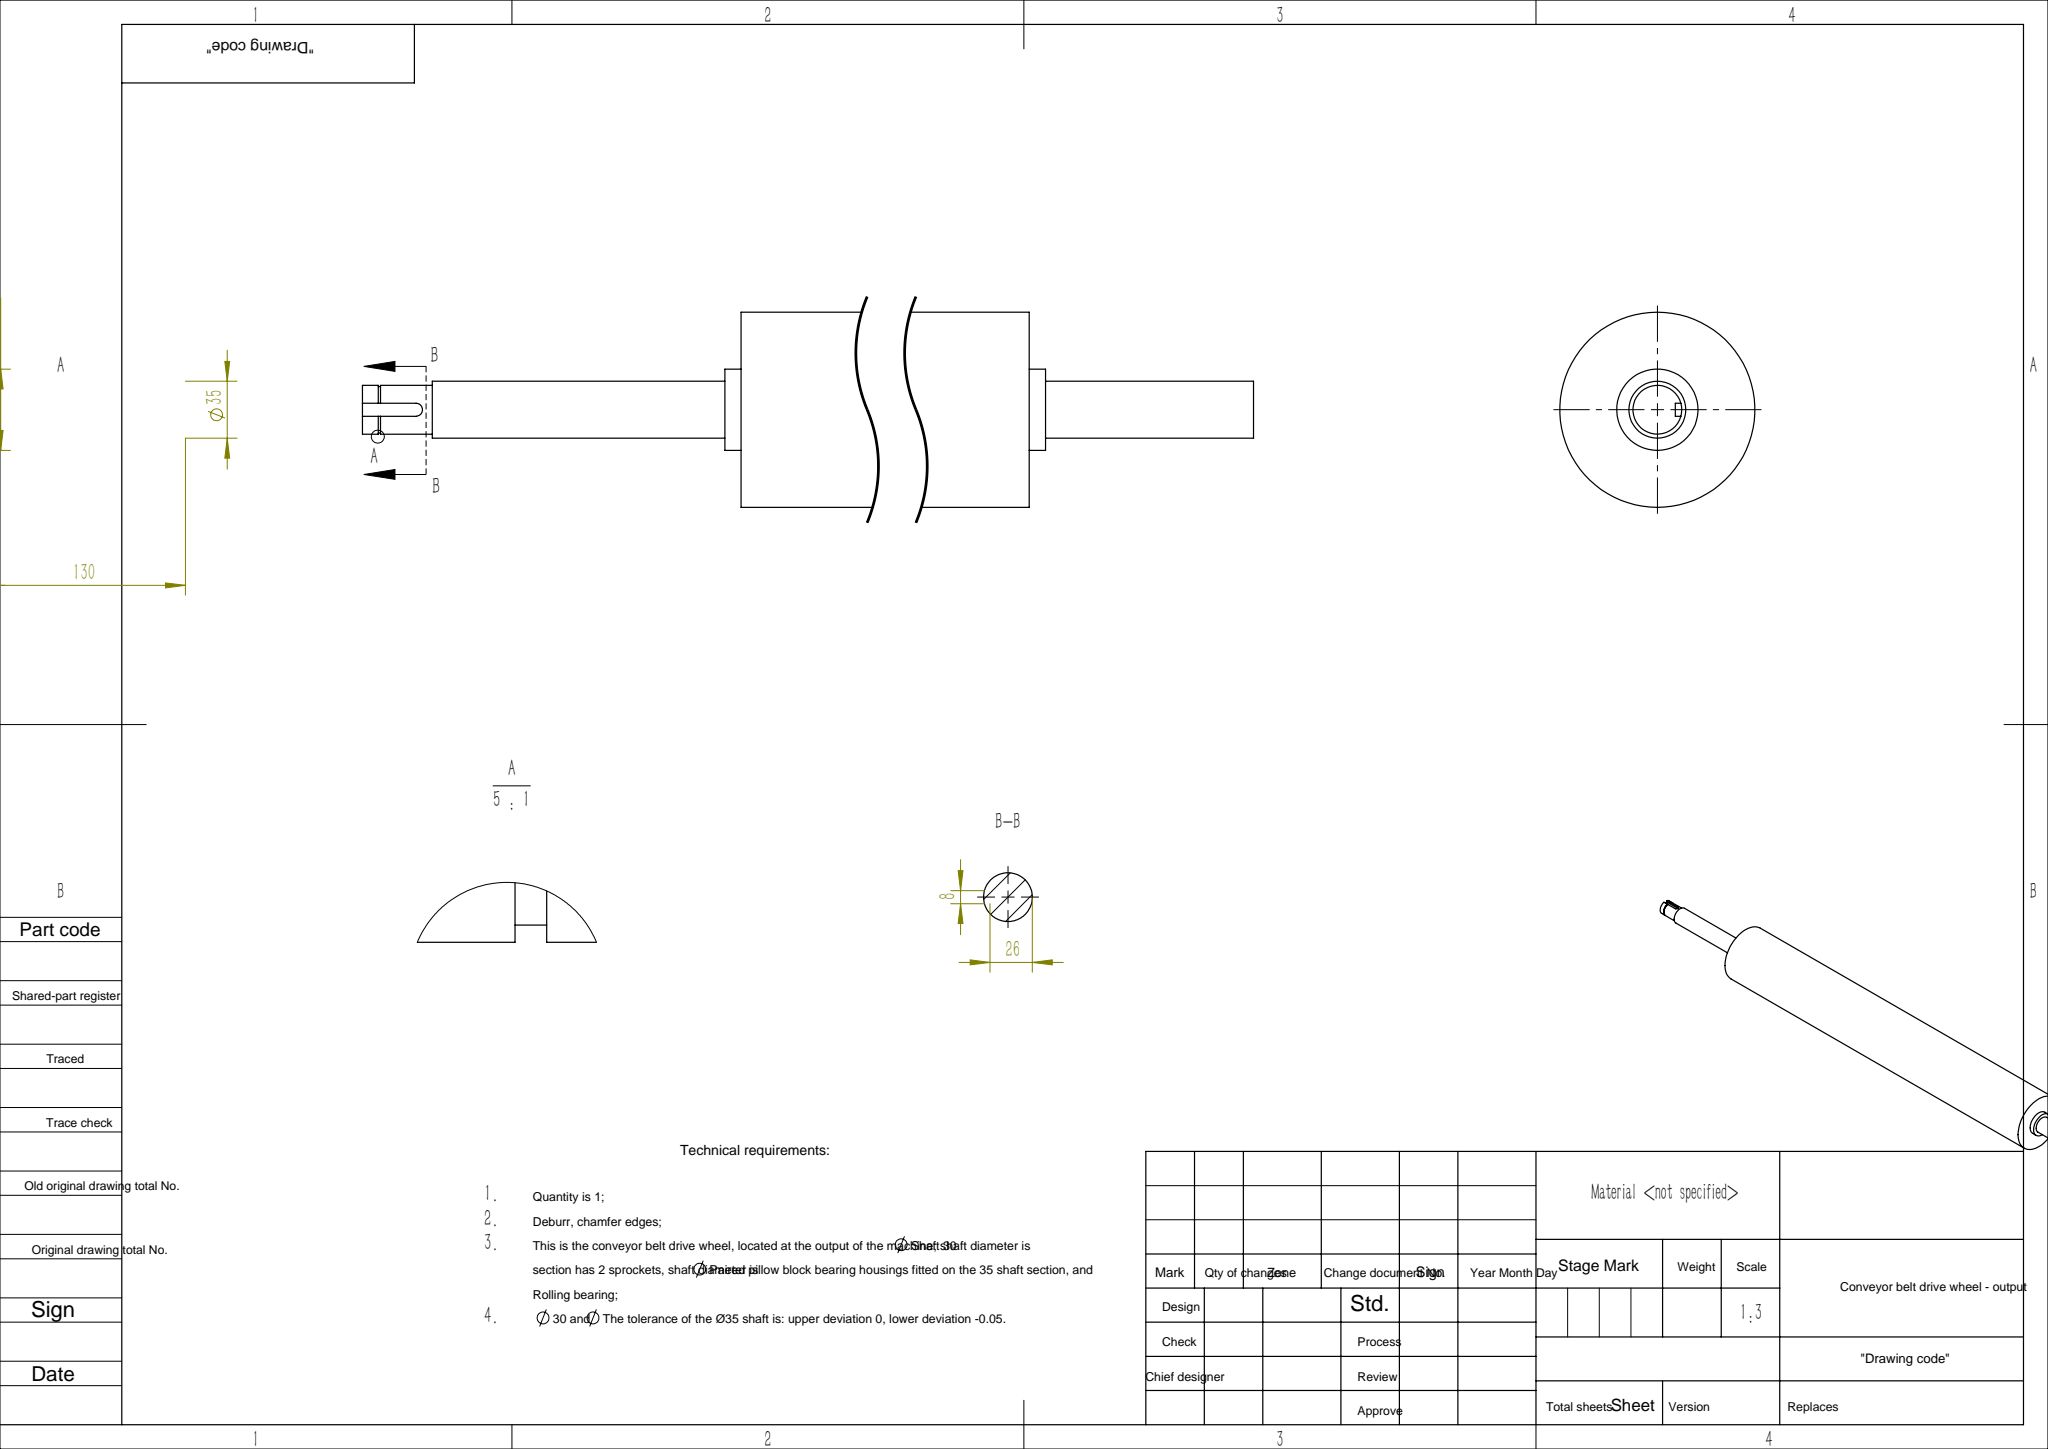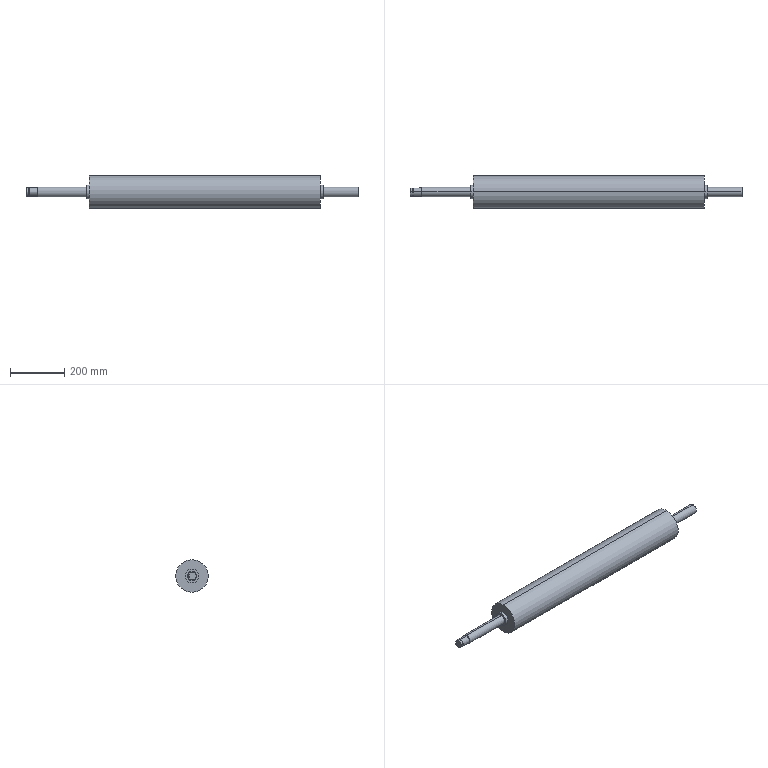Part | SolidWorks | features ICE 2, Revolution 1 | 1 solid | 31 faces | box 1221 x 120 x 120 mm | volume 9978087 mm3 | cylinder 19 | plane 12 | commonest cylinder face diameters 30 x5 35 x4 50 x4 28.6 x3 120 x2 8 x1
STEP:
#1=CARTESIAN_POINT('',(11.1,13.729,-4.));
#2=VERTEX_POINT('',#1);
#3=CARTESIAN_POINT('',(11.1,0.,-14.3));
#4=VERTEX_POINT('',#3);
#5=CARTESIAN_POINT('',(11.1,0.,0.));
#6=DIRECTION('',(-1.,0.,0.));
#7=DIRECTION('',(0.,0.,1.));
#8=AXIS2_PLACEMENT_3D('',#5,#6,#7);
#9=CIRCLE('',#8,14.3);
#10=EDGE_CURVE('',#2,#4,#9,.T.);
#11=ORIENTED_EDGE('',*,*,#10,.T.);
#12=CARTESIAN_POINT('',(9.8,0.,-14.3));
#13=VERTEX_POINT('',#12);
#14=CARTESIAN_POINT('',(11.1,0.,-14.3));
#15=DIRECTION('',(-1.,0.,0.));
#16=VECTOR('',#15,1000.);
#17=LINE('',#14,#16);
#18=EDGE_CURVE('',#4,#13,#17,.T.);
#19=ORIENTED_EDGE('',*,*,#18,.T.);
#20=CARTESIAN_POINT('',(9.8,13.729,-4.));
#21=VERTEX_POINT('',#20);
#22=CARTESIAN_POINT('',(9.8,0.,0.));
#23=DIRECTION('',(-1.,0.,0.));
#24=DIRECTION('',(0.,0.,1.));
#25=AXIS2_PLACEMENT_3D('',#22,#23,#24);
#26=CIRCLE('',#25,14.3);
#27=EDGE_CURVE('',#21,#13,#26,.T.);
#28=ORIENTED_EDGE('',*,*,#27,.F.);
#29=CARTESIAN_POINT('',(11.1,13.729,-4.));
#30=DIRECTION('',(1.,0.,0.));
#31=VECTOR('',#30,1000.);
#32=LINE('',#29,#31);
#33=EDGE_CURVE('',#21,#2,#32,.T.);
#34=ORIENTED_EDGE('',*,*,#33,.T.);
#35=EDGE_LOOP('',(#11,#19,#28,#34));
#36=FACE_OUTER_BOUND('',#35,.T.);
#37=CARTESIAN_POINT('',(11.1,0.,0.));
#38=DIRECTION('',(-1.,0.,0.));
#39=DIRECTION('',(0.,0.,1.));
#40=AXIS2_PLACEMENT_3D('',#37,#38,#39);
#41=CYLINDRICAL_SURFACE('',#40,14.3);
#42=ADVANCED_FACE('',(#36),#41,.T.);
#43=ORIENTED_EDGE('',*,*,#18,.F.);
#44=CARTESIAN_POINT('',(11.1,0.,14.3));
#45=VERTEX_POINT('',#44);
#46=CARTESIAN_POINT('',(11.1,0.,0.));
#47=DIRECTION('',(-1.,0.,0.));
#48=DIRECTION('',(0.,0.,1.));
#49=AXIS2_PLACEMENT_3D('',#46,#47,#48);
#50=CIRCLE('',#49,14.3);
#51=EDGE_CURVE('',#4,#45,#50,.T.);
#52=ORIENTED_EDGE('',*,*,#51,.T.);
#53=CARTESIAN_POINT('',(9.8,0.,14.3));
#54=VERTEX_POINT('',#53);
#55=CARTESIAN_POINT('',(11.1,0.,14.3));
#56=DIRECTION('',(-1.,0.,0.));
#57=VECTOR('',#56,1000.);
#58=LINE('',#55,#57);
#59=EDGE_CURVE('',#45,#54,#58,.T.);
#60=ORIENTED_EDGE('',*,*,#59,.T.);
#61=CARTESIAN_POINT('',(9.8,0.,0.));
#62=DIRECTION('',(-1.,0.,0.));
#63=DIRECTION('',(0.,0.,1.));
#64=AXIS2_PLACEMENT_3D('',#61,#62,#63);
#65=CIRCLE('',#64,14.3);
#66=EDGE_CURVE('',#13,#54,#65,.T.);
#67=ORIENTED_EDGE('',*,*,#66,.F.);
#68=EDGE_LOOP('',(#43,#52,#60,#67));
#69=FACE_OUTER_BOUND('',#68,.T.);
#70=CARTESIAN_POINT('',(11.1,0.,0.));
#71=DIRECTION('',(-1.,0.,0.));
#72=DIRECTION('',(0.,0.,1.));
#73=AXIS2_PLACEMENT_3D('',#70,#71,#72);
#74=CYLINDRICAL_SURFACE('',#73,14.3);
#75=ADVANCED_FACE('',(#69),#74,.T.);
#76=CARTESIAN_POINT('',(1221.,0.,17.5));
#77=VERTEX_POINT('',#76);
#78=CARTESIAN_POINT('',(1221.,0.,-17.5));
#79=VERTEX_POINT('',#78);
#80=CARTESIAN_POINT('',(1221.,0.,0.));
#81=DIRECTION('',(-1.,0.,0.));
#82=DIRECTION('',(0.,0.,1.));
#83=AXIS2_PLACEMENT_3D('',#80,#81,#82);
#84=CIRCLE('',#83,17.5);
#85=EDGE_CURVE('',#77,#79,#84,.T.);
#86=ORIENTED_EDGE('',*,*,#85,.T.);
#87=CARTESIAN_POINT('',(1093.,0.,-17.5));
#88=VERTEX_POINT('',#87);
#89=CARTESIAN_POINT('',(0.,0.,-17.5));
#90=DIRECTION('',(-1.,0.,0.));
#91=VECTOR('',#90,1000.);
#92=LINE('',#89,#91);
#93=EDGE_CURVE('',#79,#88,#92,.T.);
#94=ORIENTED_EDGE('',*,*,#93,.T.);
#95=CARTESIAN_POINT('',(1093.,0.,17.5));
#96=VERTEX_POINT('',#95);
#97=CARTESIAN_POINT('',(1093.,0.,0.));
#98=DIRECTION('',(-1.,0.,0.));
#99=DIRECTION('',(0.,0.,1.));
#100=AXIS2_PLACEMENT_3D('',#97,#98,#99);
#101=CIRCLE('',#100,17.5);
#102=EDGE_CURVE('',#96,#88,#101,.T.);
#103=ORIENTED_EDGE('',*,*,#102,.F.);
#104=CARTESIAN_POINT('',(0.,0.,17.5));
#105=DIRECTION('',(-1.,0.,0.));
#106=VECTOR('',#105,1000.);
#107=LINE('',#104,#106);
#108=EDGE_CURVE('',#77,#96,#107,.T.);
#109=ORIENTED_EDGE('',*,*,#108,.F.);
#110=EDGE_LOOP('',(#86,#94,#103,#109));
#111=FACE_OUTER_BOUND('',#110,.T.);
#112=CARTESIAN_POINT('',(0.,0.,0.));
#113=DIRECTION('',(-1.,0.,0.));
#114=DIRECTION('',(0.,0.,1.));
#115=AXIS2_PLACEMENT_3D('',#112,#113,#114);
#116=CYLINDRICAL_SURFACE('',#115,17.5);
#117=ADVANCED_FACE('',(#111),#116,.T.);
#118=CARTESIAN_POINT('',(1093.,0.,25.));
#119=VERTEX_POINT('',#118);
#120=CARTESIAN_POINT('',(1093.,0.,-25.));
#121=VERTEX_POINT('',#120);
#122=CARTESIAN_POINT('',(1093.,0.,0.));
#123=DIRECTION('',(-1.,0.,0.));
#124=DIRECTION('',(0.,0.,1.));
#125=AXIS2_PLACEMENT_3D('',#122,#123,#124);
#126=CIRCLE('',#125,25.);
#127=EDGE_CURVE('',#119,#121,#126,.T.);
#128=ORIENTED_EDGE('',*,*,#127,.T.);
#129=CARTESIAN_POINT('',(1083.,0.,-25.));
#130=VERTEX_POINT('',#129);
#131=CARTESIAN_POINT('',(0.,0.,-25.));
#132=DIRECTION('',(-1.,0.,0.));
#133=VECTOR('',#132,1000.);
#134=LINE('',#131,#133);
#135=EDGE_CURVE('',#121,#130,#134,.T.);
#136=ORIENTED_EDGE('',*,*,#135,.T.);
#137=CARTESIAN_POINT('',(1083.,0.,25.));
#138=VERTEX_POINT('',#137);
#139=CARTESIAN_POINT('',(1083.,0.,0.));
#140=DIRECTION('',(-1.,0.,0.));
#141=DIRECTION('',(0.,0.,1.));
#142=AXIS2_PLACEMENT_3D('',#139,#140,#141);
#143=CIRCLE('',#142,25.);
#144=EDGE_CURVE('',#138,#130,#143,.T.);
#145=ORIENTED_EDGE('',*,*,#144,.F.);
#146=CARTESIAN_POINT('',(0.,0.,25.));
#147=DIRECTION('',(-1.,0.,0.));
#148=VECTOR('',#147,1000.);
#149=LINE('',#146,#148);
#150=EDGE_CURVE('',#119,#138,#149,.T.);
#151=ORIENTED_EDGE('',*,*,#150,.F.);
#152=EDGE_LOOP('',(#128,#136,#145,#151));
#153=FACE_OUTER_BOUND('',#152,.T.);
#154=CARTESIAN_POINT('',(0.,0.,0.));
#155=DIRECTION('',(-1.,0.,0.));
#156=DIRECTION('',(0.,0.,1.));
#157=AXIS2_PLACEMENT_3D('',#154,#155,#156);
#158=CYLINDRICAL_SURFACE('',#157,25.);
#159=ADVANCED_FACE('',(#153),#158,.T.);
#160=CARTESIAN_POINT('',(1083.,0.,60.));
#161=VERTEX_POINT('',#160);
#162=CARTESIAN_POINT('',(1083.,0.,-60.));
#163=VERTEX_POINT('',#162);
#164=CARTESIAN_POINT('',(1083.,0.,0.));
#165=DIRECTION('',(-1.,0.,0.));
#166=DIRECTION('',(0.,0.,1.));
#167=AXIS2_PLACEMENT_3D('',#164,#165,#166);
#168=CIRCLE('',#167,60.);
#169=EDGE_CURVE('',#161,#163,#168,.T.);
#170=ORIENTED_EDGE('',*,*,#169,.T.);
#171=CARTESIAN_POINT('',(233.,0.,-60.));
#172=VERTEX_POINT('',#171);
#173=CARTESIAN_POINT('',(0.,0.,-60.));
#174=DIRECTION('',(-1.,0.,0.));
#175=VECTOR('',#174,1000.);
#176=LINE('',#173,#175);
#177=EDGE_CURVE('',#163,#172,#176,.T.);
#178=ORIENTED_EDGE('',*,*,#177,.T.);
#179=CARTESIAN_POINT('',(233.,0.,60.));
#180=VERTEX_POINT('',#179);
#181=CARTESIAN_POINT('',(233.,0.,0.));
#182=DIRECTION('',(-1.,0.,0.));
#183=DIRECTION('',(0.,0.,1.));
#184=AXIS2_PLACEMENT_3D('',#181,#182,#183);
#185=CIRCLE('',#184,60.);
#186=EDGE_CURVE('',#180,#172,#185,.T.);
#187=ORIENTED_EDGE('',*,*,#186,.F.);
#188=CARTESIAN_POINT('',(0.,0.,60.));
#189=DIRECTION('',(-1.,0.,0.));
#190=VECTOR('',#189,1000.);
#191=LINE('',#188,#190);
#192=EDGE_CURVE('',#161,#180,#191,.T.);
#193=ORIENTED_EDGE('',*,*,#192,.F.);
#194=EDGE_LOOP('',(#170,#178,#187,#193));
#195=FACE_OUTER_BOUND('',#194,.T.);
#196=CARTESIAN_POINT('',(0.,0.,0.));
#197=DIRECTION('',(-1.,0.,0.));
#198=DIRECTION('',(0.,0.,1.));
#199=AXIS2_PLACEMENT_3D('',#196,#197,#198);
#200=CYLINDRICAL_SURFACE('',#199,60.);
#201=ADVANCED_FACE('',(#195),#200,.T.);
#202=CARTESIAN_POINT('',(233.,0.,25.));
#203=VERTEX_POINT('',#202);
#204=CARTESIAN_POINT('',(233.,0.,-25.));
#205=VERTEX_POINT('',#204);
#206=CARTESIAN_POINT('',(233.,0.,0.));
#207=DIRECTION('',(-1.,0.,0.));
#208=DIRECTION('',(0.,0.,1.));
#209=AXIS2_PLACEMENT_3D('',#206,#207,#208);
#210=CIRCLE('',#209,25.);
#211=EDGE_CURVE('',#203,#205,#210,.T.);
#212=ORIENTED_EDGE('',*,*,#211,.T.);
#213=CARTESIAN_POINT('',(223.,0.,-25.));
#214=VERTEX_POINT('',#213);
#215=CARTESIAN_POINT('',(0.,0.,-25.));
#216=DIRECTION('',(-1.,0.,0.));
#217=VECTOR('',#216,1000.);
#218=LINE('',#215,#217);
#219=EDGE_CURVE('',#205,#214,#218,.T.);
#220=ORIENTED_EDGE('',*,*,#219,.T.);
#221=CARTESIAN_POINT('',(223.,0.,25.));
#222=VERTEX_POINT('',#221);
#223=CARTESIAN_POINT('',(223.,0.,0.));
#224=DIRECTION('',(-1.,0.,0.));
#225=DIRECTION('',(0.,0.,1.));
#226=AXIS2_PLACEMENT_3D('',#223,#224,#225);
#227=CIRCLE('',#226,25.);
#228=EDGE_CURVE('',#222,#214,#227,.T.);
#229=ORIENTED_EDGE('',*,*,#228,.F.);
#230=CARTESIAN_POINT('',(0.,0.,25.));
#231=DIRECTION('',(-1.,0.,0.));
#232=VECTOR('',#231,1000.);
#233=LINE('',#230,#232);
#234=EDGE_CURVE('',#203,#222,#233,.T.);
#235=ORIENTED_EDGE('',*,*,#234,.F.);
#236=EDGE_LOOP('',(#212,#220,#229,#235));
#237=FACE_OUTER_BOUND('',#236,.T.);
#238=CARTESIAN_POINT('',(0.,0.,0.));
#239=DIRECTION('',(-1.,0.,0.));
#240=DIRECTION('',(0.,0.,1.));
#241=AXIS2_PLACEMENT_3D('',#238,#239,#240);
#242=CYLINDRICAL_SURFACE('',#241,25.);
#243=ADVANCED_FACE('',(#237),#242,.T.);
#244=CARTESIAN_POINT('',(223.,0.,17.5));
#245=VERTEX_POINT('',#244);
#246=CARTESIAN_POINT('',(223.,0.,-17.5));
#247=VERTEX_POINT('',#246);
#248=CARTESIAN_POINT('',(223.,0.,0.));
#249=DIRECTION('',(-1.,0.,0.));
#250=DIRECTION('',(0.,0.,1.));
#251=AXIS2_PLACEMENT_3D('',#248,#249,#250);
#252=CIRCLE('',#251,17.5);
#253=EDGE_CURVE('',#245,#247,#252,.T.);
#254=ORIENTED_EDGE('',*,*,#253,.T.);
#255=CARTESIAN_POINT('',(43.,0.,-17.5));
#256=VERTEX_POINT('',#255);
#257=CARTESIAN_POINT('',(0.,0.,-17.5));
#258=DIRECTION('',(-1.,0.,0.));
#259=VECTOR('',#258,1000.);
#260=LINE('',#257,#259);
#261=EDGE_CURVE('',#247,#256,#260,.T.);
#262=ORIENTED_EDGE('',*,*,#261,.T.);
#263=CARTESIAN_POINT('',(43.,0.,17.5));
#264=VERTEX_POINT('',#263);
#265=CARTESIAN_POINT('',(43.,0.,0.));
#266=DIRECTION('',(-1.,0.,0.));
#267=DIRECTION('',(0.,0.,1.));
#268=AXIS2_PLACEMENT_3D('',#265,#266,#267);
#269=CIRCLE('',#268,17.5);
#270=EDGE_CURVE('',#264,#256,#269,.T.);
#271=ORIENTED_EDGE('',*,*,#270,.F.);
#272=CARTESIAN_POINT('',(0.,0.,17.5));
#273=DIRECTION('',(-1.,0.,0.));
#274=VECTOR('',#273,1000.);
#275=LINE('',#272,#274);
#276=EDGE_CURVE('',#245,#264,#275,.T.);
#277=ORIENTED_EDGE('',*,*,#276,.F.);
#278=EDGE_LOOP('',(#254,#262,#271,#277));
#279=FACE_OUTER_BOUND('',#278,.T.);
#280=CARTESIAN_POINT('',(0.,0.,0.));
#281=DIRECTION('',(-1.,0.,0.));
#282=DIRECTION('',(0.,0.,1.));
#283=AXIS2_PLACEMENT_3D('',#280,#281,#282);
#284=CYLINDRICAL_SURFACE('',#283,17.5);
#285=ADVANCED_FACE('',(#279),#284,.T.);
#286=CARTESIAN_POINT('',(9.8,14.457,-4.));
#287=VERTEX_POINT('',#286);
#288=CARTESIAN_POINT('',(9.8,0.,-15.));
#289=VERTEX_POINT('',#288);
#290=CARTESIAN_POINT('',(9.8,0.,0.));
#291=DIRECTION('',(-1.,0.,0.));
#292=DIRECTION('',(0.,0.,1.));
#293=AXIS2_PLACEMENT_3D('',#290,#291,#292);
#294=CIRCLE('',#293,15.);
#295=EDGE_CURVE('',#287,#289,#294,.T.);
#296=ORIENTED_EDGE('',*,*,#295,.T.);
#297=CARTESIAN_POINT('',(0.,0.,-15.));
#298=VERTEX_POINT('',#297);
#299=CARTESIAN_POINT('',(0.,0.,-15.));
#300=DIRECTION('',(-1.,0.,0.));
#301=VECTOR('',#300,1000.);
#302=LINE('',#299,#301);
#303=EDGE_CURVE('',#289,#298,#302,.T.);
#304=ORIENTED_EDGE('',*,*,#303,.T.);
#305=CARTESIAN_POINT('',(0.,14.457,-4.));
#306=VERTEX_POINT('',#305);
#307=CARTESIAN_POINT('',(0.,0.,0.));
#308=DIRECTION('',(-1.,0.,0.));
#309=DIRECTION('',(0.,0.,1.));
#310=AXIS2_PLACEMENT_3D('',#307,#308,#309);
#311=CIRCLE('',#310,15.);
#312=EDGE_CURVE('',#306,#298,#311,.T.);
#313=ORIENTED_EDGE('',*,*,#312,.F.);
#314=CARTESIAN_POINT('',(0.,14.457,-4.));
#315=DIRECTION('',(1.,0.,0.));
#316=VECTOR('',#315,1000.);
#317=LINE('',#314,#316);
#318=EDGE_CURVE('',#306,#287,#317,.T.);
#319=ORIENTED_EDGE('',*,*,#318,.T.);
#320=EDGE_LOOP('',(#296,#304,#313,#319));
#321=FACE_OUTER_BOUND('',#320,.T.);
#322=CARTESIAN_POINT('',(0.,0.,0.));
#323=DIRECTION('',(-1.,0.,0.));
#324=DIRECTION('',(0.,0.,1.));
#325=AXIS2_PLACEMENT_3D('',#322,#323,#324);
#326=CYLINDRICAL_SURFACE('',#325,15.);
#327=ADVANCED_FACE('',(#321),#326,.T.);
#328=ORIENTED_EDGE('',*,*,#303,.F.);
#329=CARTESIAN_POINT('',(9.8,0.,15.));
#330=VERTEX_POINT('',#329);
#331=CARTESIAN_POINT('',(9.8,0.,0.));
#332=DIRECTION('',(-1.,0.,0.));
#333=DIRECTION('',(0.,0.,1.));
#334=AXIS2_PLACEMENT_3D('',#331,#332,#333);
#335=CIRCLE('',#334,15.);
#336=EDGE_CURVE('',#289,#330,#335,.T.);
#337=ORIENTED_EDGE('',*,*,#336,.T.);
#338=CARTESIAN_POINT('',(0.,0.,15.));
#339=VERTEX_POINT('',#338);
#340=CARTESIAN_POINT('',(0.,0.,15.));
#341=DIRECTION('',(-1.,0.,0.));
#342=VECTOR('',#341,1000.);
#343=LINE('',#340,#342);
#344=EDGE_CURVE('',#330,#339,#343,.T.);
#345=ORIENTED_EDGE('',*,*,#344,.T.);
#346=CARTESIAN_POINT('',(0.,0.,0.));
#347=DIRECTION('',(-1.,0.,0.));
#348=DIRECTION('',(0.,0.,1.));
#349=AXIS2_PLACEMENT_3D('',#346,#347,#348);
#350=CIRCLE('',#349,15.);
#351=EDGE_CURVE('',#298,#339,#350,.T.);
#352=ORIENTED_EDGE('',*,*,#351,.F.);
#353=EDGE_LOOP('',(#328,#337,#345,#352));
#354=FACE_OUTER_BOUND('',#353,.T.);
#355=CARTESIAN_POINT('',(0.,0.,0.));
#356=DIRECTION('',(-1.,0.,0.));
#357=DIRECTION('',(0.,0.,1.));
#358=AXIS2_PLACEMENT_3D('',#355,#356,#357);
#359=CYLINDRICAL_SURFACE('',#358,15.);
#360=ADVANCED_FACE('',(#354),#359,.T.);
#361=CARTESIAN_POINT('',(43.,0.,15.));
#362=VERTEX_POINT('',#361);
#363=CARTESIAN_POINT('',(43.,0.,-15.));
#364=VERTEX_POINT('',#363);
#365=CARTESIAN_POINT('',(43.,0.,0.));
#366=DIRECTION('',(-1.,0.,0.));
#367=DIRECTION('',(0.,0.,1.));
#368=AXIS2_PLACEMENT_3D('',#365,#366,#367);
#369=CIRCLE('',#368,15.);
#370=EDGE_CURVE('',#362,#364,#369,.T.);
#371=ORIENTED_EDGE('',*,*,#370,.T.);
#372=CARTESIAN_POINT('',(11.1,0.,-15.));
#373=VERTEX_POINT('',#372);
#374=CARTESIAN_POINT('',(0.,0.,-15.));
#375=DIRECTION('',(-1.,0.,0.));
#376=VECTOR('',#375,1000.);
#377=LINE('',#374,#376);
#378=EDGE_CURVE('',#364,#373,#377,.T.);
#379=ORIENTED_EDGE('',*,*,#378,.T.);
#380=CARTESIAN_POINT('',(11.1,14.457,-4.));
#381=VERTEX_POINT('',#380);
#382=CARTESIAN_POINT('',(11.1,0.,0.));
#383=DIRECTION('',(-1.,0.,0.));
#384=DIRECTION('',(0.,0.,1.));
#385=AXIS2_PLACEMENT_3D('',#382,#383,#384);
#386=CIRCLE('',#385,15.);
#387=EDGE_CURVE('',#381,#373,#386,.T.);
#388=ORIENTED_EDGE('',*,*,#387,.F.);
#389=CARTESIAN_POINT('',(33.,14.457,-4.));
#390=VERTEX_POINT('',#389);
#391=CARTESIAN_POINT('',(0.,14.457,-4.));
#392=DIRECTION('',(1.,0.,0.));
#393=VECTOR('',#392,1000.);
#394=LINE('',#391,#393);
#395=EDGE_CURVE('',#381,#390,#394,.T.);
#396=ORIENTED_EDGE('',*,*,#395,.T.);
#397=CARTESIAN_POINT('',(33.,14.457,4.));
#398=VERTEX_POINT('',#397);
#399=CARTESIAN_POINT('',(33.,14.457,-4.));
#400=CARTESIAN_POINT('',(33.266,14.457,-4.));
#401=CARTESIAN_POINT('',(33.526,14.464,-3.974));
#402=CARTESIAN_POINT('',(34.039,14.492,-3.872));
#403=CARTESIAN_POINT('',(34.294,14.513,-3.794));
#404=CARTESIAN_POINT('',(34.777,14.564,-3.593));
#405=CARTESIAN_POINT('',(35.007,14.594,-3.47));
#406=CARTESIAN_POINT('',(35.44,14.66,-3.18));
#407=CARTESIAN_POINT('',(35.645,14.696,-3.012));
#408=CARTESIAN_POINT('',(36.012,14.766,-2.645));
#409=CARTESIAN_POINT('',(36.177,14.801,-2.444));
#410=CARTESIAN_POINT('',(36.47,14.867,-2.008));
#411=CARTESIAN_POINT('',(36.593,14.896,-1.777));
#412=CARTESIAN_POINT('',(36.793,14.946,-1.296));
#413=CARTESIAN_POINT('',(36.871,14.966,-1.043));
#414=CARTESIAN_POINT('',(36.974,14.993,-0.5261));
#415=CARTESIAN_POINT('',(37.,15.,-0.2658));
#416=CARTESIAN_POINT('',(37.,15.,0.2585));
#417=CARTESIAN_POINT('',(36.974,14.993,0.5249));
#418=CARTESIAN_POINT('',(36.872,14.966,1.039));
#419=CARTESIAN_POINT('',(36.796,14.947,1.289));
#420=CARTESIAN_POINT('',(36.494,14.872,2.017));
#421=CARTESIAN_POINT('',(36.199,14.802,2.457));
#422=CARTESIAN_POINT('',(35.645,14.696,3.012));
#423=CARTESIAN_POINT('',(35.444,14.66,3.177));
#424=CARTESIAN_POINT('',(35.012,14.595,3.467));
#425=CARTESIAN_POINT('',(34.778,14.564,3.593));
#426=CARTESIAN_POINT('',(34.296,14.513,3.793));
#427=CARTESIAN_POINT('',(34.046,14.492,3.87));
#428=CARTESIAN_POINT('',(33.531,14.464,3.973));
#429=CARTESIAN_POINT('',(33.266,14.457,4.));
#430=CARTESIAN_POINT('',(33.,14.457,4.));
#431=B_SPLINE_CURVE_WITH_KNOTS('',3,(#399,#400,#401,#402,#403,#404,#405,#406,#407,#408,#409,#410,#411,#412,#413,#414,#415,#416,#417,#418,#419,#420,#421,#422,#423,#424,#425,#426,#427,#428,#429,#430),.UNSPECIFIED.,.F.,.F.,(4,2,2,2,2,2,2,2,2,2,2,2,2,2,2,4),(0.,0.0007849,0.00157,0.002355,0.00314,0.003925,0.00471,0.005494,0.006279,0.007064,0.007849,0.009419,0.0102,0.01099,0.01177,0.01256),.UNSPECIFIED.);
#432=EDGE_CURVE('',#390,#398,#431,.T.);
#433=ORIENTED_EDGE('',*,*,#432,.T.);
#434=CARTESIAN_POINT('',(11.1,14.457,4.));
#435=VERTEX_POINT('',#434);
#436=CARTESIAN_POINT('',(0.,14.457,4.));
#437=DIRECTION('',(-1.,0.,0.));
#438=VECTOR('',#437,1000.);
#439=LINE('',#436,#438);
#440=EDGE_CURVE('',#398,#435,#439,.T.);
#441=ORIENTED_EDGE('',*,*,#440,.T.);
#442=CARTESIAN_POINT('',(11.1,0.,15.));
#443=VERTEX_POINT('',#442);
#444=CARTESIAN_POINT('',(11.1,0.,0.));
#445=DIRECTION('',(-1.,0.,0.));
#446=DIRECTION('',(0.,0.,1.));
#447=AXIS2_PLACEMENT_3D('',#444,#445,#446);
#448=CIRCLE('',#447,15.);
#449=EDGE_CURVE('',#443,#435,#448,.T.);
#450=ORIENTED_EDGE('',*,*,#449,.F.);
#451=CARTESIAN_POINT('',(0.,0.,15.));
#452=DIRECTION('',(-1.,0.,0.));
#453=VECTOR('',#452,1000.);
#454=LINE('',#451,#453);
#455=EDGE_CURVE('',#362,#443,#454,.T.);
#456=ORIENTED_EDGE('',*,*,#455,.F.);
#457=EDGE_LOOP('',(#371,#379,#388,#396,#433,#441,#450,#456));
#458=FACE_OUTER_BOUND('',#457,.T.);
#459=CARTESIAN_POINT('',(0.,0.,0.));
#460=DIRECTION('',(-1.,0.,0.));
#461=DIRECTION('',(0.,0.,1.));
#462=AXIS2_PLACEMENT_3D('',#459,#460,#461);
#463=CYLINDRICAL_SURFACE('',#462,15.);
#464=ADVANCED_FACE('',(#458),#463,.T.);
#465=ORIENTED_EDGE('',*,*,#378,.F.);
#466=CARTESIAN_POINT('',(43.,0.,0.));
#467=DIRECTION('',(-1.,0.,0.));
#468=DIRECTION('',(0.,0.,1.));
#469=AXIS2_PLACEMENT_3D('',#466,#467,#468);
#470=CIRCLE('',#469,15.);
#471=EDGE_CURVE('',#364,#362,#470,.T.);
#472=ORIENTED_EDGE('',*,*,#471,.T.);
#473=ORIENTED_EDGE('',*,*,#455,.T.);
#474=CARTESIAN_POINT('',(11.1,0.,0.));
#475=DIRECTION('',(-1.,0.,0.));
#476=DIRECTION('',(0.,0.,1.));
#477=AXIS2_PLACEMENT_3D('',#474,#475,#476);
#478=CIRCLE('',#477,15.);
#479=EDGE_CURVE('',#373,#443,#478,.T.);
#480=ORIENTED_EDGE('',*,*,#479,.F.);
#481=EDGE_LOOP('',(#465,#472,#473,#480));
#482=FACE_OUTER_BOUND('',#481,.T.);
#483=CARTESIAN_POINT('',(0.,0.,0.));
#484=DIRECTION('',(-1.,0.,0.));
#485=DIRECTION('',(0.,0.,1.));
#486=AXIS2_PLACEMENT_3D('',#483,#484,#485);
#487=CYLINDRICAL_SURFACE('',#486,15.);
#488=ADVANCED_FACE('',(#482),#487,.T.);
#489=CARTESIAN_POINT('',(11.1,13.729,4.));
#490=VERTEX_POINT('',#489);
#491=CARTESIAN_POINT('',(11.1,11.,4.));
#492=DIRECTION('',(0.,-1.,0.));
#493=VECTOR('',#492,1000.);
#494=LINE('',#491,#493);
#495=EDGE_CURVE('',#435,#490,#494,.T.);
#496=ORIENTED_EDGE('',*,*,#495,.F.);
#497=ORIENTED_EDGE('',*,*,#440,.F.);
#498=CARTESIAN_POINT('',(33.,11.,4.));
#499=VERTEX_POINT('',#498);
#500=CARTESIAN_POINT('',(33.,11.,4.));
#501=DIRECTION('',(0.,1.,0.));
#502=VECTOR('',#501,1000.);
#503=LINE('',#500,#502);
#504=EDGE_CURVE('',#499,#398,#503,.T.);
#505=ORIENTED_EDGE('',*,*,#504,.F.);
#506=CARTESIAN_POINT('',(0.,11.,4.));
#507=VERTEX_POINT('',#506);
#508=CARTESIAN_POINT('',(-10.,11.,4.));
#509=DIRECTION('',(1.,0.,0.));
#510=VECTOR('',#509,1000.);
#511=LINE('',#508,#510);
#512=EDGE_CURVE('',#507,#499,#511,.T.);
#513=ORIENTED_EDGE('',*,*,#512,.F.);
#514=CARTESIAN_POINT('',(0.,14.457,4.));
#515=VERTEX_POINT('',#514);
#516=CARTESIAN_POINT('',(0.,0.,4.));
#517=DIRECTION('',(0.,-1.,0.));
#518=VECTOR('',#517,1000.);
#519=LINE('',#516,#518);
#520=EDGE_CURVE('',#515,#507,#519,.T.);
#521=ORIENTED_EDGE('',*,*,#520,.F.);
#522=CARTESIAN_POINT('',(9.8,14.457,4.));
#523=VERTEX_POINT('',#522);
#524=CARTESIAN_POINT('',(0.,14.457,4.));
#525=DIRECTION('',(-1.,0.,0.));
#526=VECTOR('',#525,1000.);
#527=LINE('',#524,#526);
#528=EDGE_CURVE('',#523,#515,#527,.T.);
#529=ORIENTED_EDGE('',*,*,#528,.F.);
#530=CARTESIAN_POINT('',(9.8,13.729,4.));
#531=VERTEX_POINT('',#530);
#532=CARTESIAN_POINT('',(9.8,11.,4.));
#533=DIRECTION('',(0.,-1.,0.));
#534=VECTOR('',#533,1000.);
#535=LINE('',#532,#534);
#536=EDGE_CURVE('',#523,#531,#535,.T.);
#537=ORIENTED_EDGE('',*,*,#536,.T.);
#538=CARTESIAN_POINT('',(11.1,13.729,4.));
#539=DIRECTION('',(-1.,0.,0.));
#540=VECTOR('',#539,1000.);
#541=LINE('',#538,#540);
#542=EDGE_CURVE('',#490,#531,#541,.T.);
#543=ORIENTED_EDGE('',*,*,#542,.F.);
#544=EDGE_LOOP('',(#496,#497,#505,#513,#521,#529,#537,#543));
#545=FACE_OUTER_BOUND('',#544,.T.);
#546=CARTESIAN_POINT('',(-10.,11.,4.));
#547=DIRECTION('',(0.,0.,1.));
#548=DIRECTION('',(1.,0.,0.));
#549=AXIS2_PLACEMENT_3D('',#546,#547,#548);
#550=PLANE('',#549);
#551=ADVANCED_FACE('',(#545),#550,.F.);
#552=CARTESIAN_POINT('',(11.1,11.,-4.));
#553=DIRECTION('',(0.,1.,0.));
#554=VECTOR('',#553,1000.);
#555=LINE('',#552,#554);
#556=EDGE_CURVE('',#2,#381,#555,.T.);
#557=ORIENTED_EDGE('',*,*,#556,.F.);
#558=ORIENTED_EDGE('',*,*,#33,.F.);
#559=CARTESIAN_POINT('',(9.8,11.,-4.));
#560=DIRECTION('',(0.,1.,0.));
#561=VECTOR('',#560,1000.);
#562=LINE('',#559,#561);
#563=EDGE_CURVE('',#21,#287,#562,.T.);
#564=ORIENTED_EDGE('',*,*,#563,.T.);
#565=ORIENTED_EDGE('',*,*,#318,.F.);
#566=CARTESIAN_POINT('',(0.,11.,-4.));
#567=VERTEX_POINT('',#566);
#568=CARTESIAN_POINT('',(0.,0.,-4.));
#569=DIRECTION('',(0.,1.,0.));
#570=VECTOR('',#569,1000.);
#571=LINE('',#568,#570);
#572=EDGE_CURVE('',#567,#306,#571,.T.);
#573=ORIENTED_EDGE('',*,*,#572,.F.);
#574=CARTESIAN_POINT('',(33.,11.,-4.));
#575=VERTEX_POINT('',#574);
#576=CARTESIAN_POINT('',(33.,11.,-4.));
#577=DIRECTION('',(-1.,0.,0.));
#578=VECTOR('',#577,1000.);
#579=LINE('',#576,#578);
#580=EDGE_CURVE('',#575,#567,#579,.T.);
#581=ORIENTED_EDGE('',*,*,#580,.F.);
#582=CARTESIAN_POINT('',(33.,11.,-4.));
#583=DIRECTION('',(0.,1.,0.));
#584=VECTOR('',#583,1000.);
#585=LINE('',#582,#584);
#586=EDGE_CURVE('',#575,#390,#585,.T.);
#587=ORIENTED_EDGE('',*,*,#586,.T.);
#588=ORIENTED_EDGE('',*,*,#395,.F.);
#589=EDGE_LOOP('',(#557,#558,#564,#565,#573,#581,#587,#588));
#590=FACE_OUTER_BOUND('',#589,.T.);
#591=CARTESIAN_POINT('',(33.,11.,-4.));
#592=DIRECTION('',(0.,0.,-1.));
#593=DIRECTION('',(-1.,0.,0.));
#594=AXIS2_PLACEMENT_3D('',#591,#592,#593);
#595=PLANE('',#594);
#596=ADVANCED_FACE('',(#590),#595,.F.);
#597=ORIENTED_EDGE('',*,*,#312,.T.);
#598=ORIENTED_EDGE('',*,*,#351,.T.);
#599=CARTESIAN_POINT('',(0.,0.,0.));
#600=DIRECTION('',(-1.,0.,0.));
#601=DIRECTION('',(0.,0.,1.));
#602=AXIS2_PLACEMENT_3D('',#599,#600,#601);
#603=CIRCLE('',#602,15.);
#604=EDGE_CURVE('',#339,#515,#603,.T.);
#605=ORIENTED_EDGE('',*,*,#604,.T.);
#606=ORIENTED_EDGE('',*,*,#520,.T.);
#607=CARTESIAN_POINT('',(0.,11.,0.));
#608=DIRECTION('',(0.,0.,1.));
#609=VECTOR('',#608,1000.);
#610=LINE('',#607,#609);
#611=EDGE_CURVE('',#567,#507,#610,.T.);
#612=ORIENTED_EDGE('',*,*,#611,.F.);
#613=ORIENTED_EDGE('',*,*,#572,.T.);
#614=EDGE_LOOP('',(#597,#598,#605,#606,#612,#613));
#615=FACE_OUTER_BOUND('',#614,.T.);
#616=CARTESIAN_POINT('',(0.,0.,0.));
#617=DIRECTION('',(1.,0.,0.));
#618=DIRECTION('',(0.,0.,-1.));
#619=AXIS2_PLACEMENT_3D('',#616,#617,#618);
#620=PLANE('',#619);
#621=ADVANCED_FACE('',(#615),#620,.F.);
#622=ORIENTED_EDGE('',*,*,#344,.F.);
#623=CARTESIAN_POINT('',(9.8,0.,0.));
#624=DIRECTION('',(-1.,0.,0.));
#625=DIRECTION('',(0.,0.,1.));
#626=AXIS2_PLACEMENT_3D('',#623,#624,#625);
#627=CIRCLE('',#626,15.);
#628=EDGE_CURVE('',#330,#523,#627,.T.);
#629=ORIENTED_EDGE('',*,*,#628,.T.);
#630=ORIENTED_EDGE('',*,*,#528,.T.);
#631=ORIENTED_EDGE('',*,*,#604,.F.);
#632=EDGE_LOOP('',(#622,#629,#630,#631));
#633=FACE_OUTER_BOUND('',#632,.T.);
#634=CARTESIAN_POINT('',(0.,0.,0.));
#635=DIRECTION('',(-1.,0.,0.));
#636=DIRECTION('',(0.,0.,1.));
#637=AXIS2_PLACEMENT_3D('',#634,#635,#636);
#638=CYLINDRICAL_SURFACE('',#637,15.);
#639=ADVANCED_FACE('',(#633),#638,.T.);
#640=ORIENTED_EDGE('',*,*,#370,.F.);
#641=ORIENTED_EDGE('',*,*,#471,.F.);
#642=EDGE_LOOP('',(#640,#641));
#643=FACE_BOUND('',#642,.T.);
#644=ORIENTED_EDGE('',*,*,#270,.T.);
#645=CARTESIAN_POINT('',(43.,0.,0.));
#646=DIRECTION('',(-1.,0.,0.));
#647=DIRECTION('',(0.,0.,1.));
#648=AXIS2_PLACEMENT_3D('',#645,#646,#647);
#649=CIRCLE('',#648,17.5);
#650=EDGE_CURVE('',#256,#264,#649,.T.);
#651=ORIENTED_EDGE('',*,*,#650,.T.);
#652=EDGE_LOOP('',(#644,#651));
#653=FACE_OUTER_BOUND('',#652,.T.);
#654=CARTESIAN_POINT('',(43.,15.,0.));
#655=DIRECTION('',(1.,0.,0.));
#656=DIRECTION('',(0.,0.,-1.));
#657=AXIS2_PLACEMENT_3D('',#654,#655,#656);
#658=PLANE('',#657);
#659=ADVANCED_FACE('',(#643,#653),#658,.F.);
#660=ORIENTED_EDGE('',*,*,#261,.F.);
#661=CARTESIAN_POINT('',(223.,0.,0.));
#662=DIRECTION('',(-1.,0.,0.));
#663=DIRECTION('',(0.,0.,1.));
#664=AXIS2_PLACEMENT_3D('',#661,#662,#663);
#665=CIRCLE('',#664,17.5);
#666=EDGE_CURVE('',#247,#245,#665,.T.);
#667=ORIENTED_EDGE('',*,*,#666,.T.);
#668=ORIENTED_EDGE('',*,*,#276,.T.);
#669=ORIENTED_EDGE('',*,*,#650,.F.);
#670=EDGE_LOOP('',(#660,#667,#668,#669));
#671=FACE_OUTER_BOUND('',#670,.T.);
#672=CARTESIAN_POINT('',(0.,0.,0.));
#673=DIRECTION('',(-1.,0.,0.));
#674=DIRECTION('',(0.,0.,1.));
#675=AXIS2_PLACEMENT_3D('',#672,#673,#674);
#676=CYLINDRICAL_SURFACE('',#675,17.5);
#677=ADVANCED_FACE('',(#671),#676,.T.);
#678=ORIENTED_EDGE('',*,*,#253,.F.);
#679=ORIENTED_EDGE('',*,*,#666,.F.);
#680=EDGE_LOOP('',(#678,#679));
#681=FACE_BOUND('',#680,.T.);
#682=ORIENTED_EDGE('',*,*,#228,.T.);
#683=CARTESIAN_POINT('',(223.,0.,0.));
#684=DIRECTION('',(-1.,0.,0.));
#685=DIRECTION('',(0.,0.,1.));
#686=AXIS2_PLACEMENT_3D('',#683,#684,#685);
#687=CIRCLE('',#686,25.);
#688=EDGE_CURVE('',#214,#222,#687,.T.);
#689=ORIENTED_EDGE('',*,*,#688,.T.);
#690=EDGE_LOOP('',(#682,#689));
#691=FACE_OUTER_BOUND('',#690,.T.);
#692=CARTESIAN_POINT('',(223.,17.5,0.));
#693=DIRECTION('',(1.,0.,0.));
#694=DIRECTION('',(0.,0.,-1.));
#695=AXIS2_PLACEMENT_3D('',#692,#693,#694);
#696=PLANE('',#695);
#697=ADVANCED_FACE('',(#681,#691),#696,.F.);
#698=ORIENTED_EDGE('',*,*,#219,.F.);
#699=CARTESIAN_POINT('',(233.,0.,0.));
#700=DIRECTION('',(-1.,0.,0.));
#701=DIRECTION('',(0.,0.,1.));
#702=AXIS2_PLACEMENT_3D('',#699,#700,#701);
#703=CIRCLE('',#702,25.);
#704=EDGE_CURVE('',#205,#203,#703,.T.);
#705=ORIENTED_EDGE('',*,*,#704,.T.);
#706=ORIENTED_EDGE('',*,*,#234,.T.);
#707=ORIENTED_EDGE('',*,*,#688,.F.);
#708=EDGE_LOOP('',(#698,#705,#706,#707));
#709=FACE_OUTER_BOUND('',#708,.T.);
#710=CARTESIAN_POINT('',(0.,0.,0.));
#711=DIRECTION('',(-1.,0.,0.));
#712=DIRECTION('',(0.,0.,1.));
#713=AXIS2_PLACEMENT_3D('',#710,#711,#712);
#714=CYLINDRICAL_SURFACE('',#713,25.);
#715=ADVANCED_FACE('',(#709),#714,.T.);
#716=ORIENTED_EDGE('',*,*,#211,.F.);
#717=ORIENTED_EDGE('',*,*,#704,.F.);
#718=EDGE_LOOP('',(#716,#717));
#719=FACE_BOUND('',#718,.T.);
#720=ORIENTED_EDGE('',*,*,#186,.T.);
#721=CARTESIAN_POINT('',(233.,0.,0.));
#722=DIRECTION('',(-1.,0.,0.));
#723=DIRECTION('',(0.,0.,1.));
#724=AXIS2_PLACEMENT_3D('',#721,#722,#723);
#725=CIRCLE('',#724,60.);
#726=EDGE_CURVE('',#172,#180,#725,.T.);
#727=ORIENTED_EDGE('',*,*,#726,.T.);
#728=EDGE_LOOP('',(#720,#727));
#729=FACE_OUTER_BOUND('',#728,.T.);
#730=CARTESIAN_POINT('',(233.,25.,0.));
#731=DIRECTION('',(1.,0.,0.));
#732=DIRECTION('',(0.,0.,-1.));
#733=AXIS2_PLACEMENT_3D('',#730,#731,#732);
#734=PLANE('',#733);
#735=ADVANCED_FACE('',(#719,#729),#734,.F.);
#736=ORIENTED_EDGE('',*,*,#177,.F.);
#737=CARTESIAN_POINT('',(1083.,0.,0.));
#738=DIRECTION('',(-1.,0.,0.));
#739=DIRECTION('',(0.,0.,1.));
#740=AXIS2_PLACEMENT_3D('',#737,#738,#739);
#741=CIRCLE('',#740,60.);
#742=EDGE_CURVE('',#163,#161,#741,.T.);
#743=ORIENTED_EDGE('',*,*,#742,.T.);
#744=ORIENTED_EDGE('',*,*,#192,.T.);
#745=ORIENTED_EDGE('',*,*,#726,.F.);
#746=EDGE_LOOP('',(#736,#743,#744,#745));
#747=FACE_OUTER_BOUND('',#746,.T.);
#748=CARTESIAN_POINT('',(0.,0.,0.));
#749=DIRECTION('',(-1.,0.,0.));
#750=DIRECTION('',(0.,0.,1.));
#751=AXIS2_PLACEMENT_3D('',#748,#749,#750);
#752=CYLINDRICAL_SURFACE('',#751,60.);
#753=ADVANCED_FACE('',(#747),#752,.T.);
#754=ORIENTED_EDGE('',*,*,#169,.F.);
#755=ORIENTED_EDGE('',*,*,#742,.F.);
#756=EDGE_LOOP('',(#754,#755));
#757=FACE_OUTER_BOUND('',#756,.T.);
#758=ORIENTED_EDGE('',*,*,#144,.T.);
#759=CARTESIAN_POINT('',(1083.,0.,0.));
#760=DIRECTION('',(-1.,0.,0.));
#761=DIRECTION('',(0.,0.,1.));
#762=AXIS2_PLACEMENT_3D('',#759,#760,#761);
#763=CIRCLE('',#762,25.);
#764=EDGE_CURVE('',#130,#138,#763,.T.);
#765=ORIENTED_EDGE('',*,*,#764,.T.);
#766=EDGE_LOOP('',(#758,#765));
#767=FACE_BOUND('',#766,.T.);
#768=CARTESIAN_POINT('',(1083.,60.,0.));
#769=DIRECTION('',(-1.,0.,0.));
#770=DIRECTION('',(0.,0.,1.));
#771=AXIS2_PLACEMENT_3D('',#768,#769,#770);
#772=PLANE('',#771);
#773=ADVANCED_FACE('',(#757,#767),#772,.F.);
#774=ORIENTED_EDGE('',*,*,#135,.F.);
#775=CARTESIAN_POINT('',(1093.,0.,0.));
#776=DIRECTION('',(-1.,0.,0.));
#777=DIRECTION('',(0.,0.,1.));
#778=AXIS2_PLACEMENT_3D('',#775,#776,#777);
#779=CIRCLE('',#778,25.);
#780=EDGE_CURVE('',#121,#119,#779,.T.);
#781=ORIENTED_EDGE('',*,*,#780,.T.);
#782=ORIENTED_EDGE('',*,*,#150,.T.);
#783=ORIENTED_EDGE('',*,*,#764,.F.);
#784=EDGE_LOOP('',(#774,#781,#782,#783));
#785=FACE_OUTER_BOUND('',#784,.T.);
#786=CARTESIAN_POINT('',(0.,0.,0.));
#787=DIRECTION('',(-1.,0.,0.));
#788=DIRECTION('',(0.,0.,1.));
#789=AXIS2_PLACEMENT_3D('',#786,#787,#788);
#790=CYLINDRICAL_SURFACE('',#789,25.);
#791=ADVANCED_FACE('',(#785),#790,.T.);
#792=ORIENTED_EDGE('',*,*,#127,.F.);
#793=ORIENTED_EDGE('',*,*,#780,.F.);
#794=EDGE_LOOP('',(#792,#793));
#795=FACE_OUTER_BOUND('',#794,.T.);
#796=ORIENTED_EDGE('',*,*,#102,.T.);
#797=CARTESIAN_POINT('',(1093.,0.,0.));
#798=DIRECTION('',(-1.,0.,0.));
#799=DIRECTION('',(0.,0.,1.));
#800=AXIS2_PLACEMENT_3D('',#797,#798,#799);
#801=CIRCLE('',#800,17.5);
#802=EDGE_CURVE('',#88,#96,#801,.T.);
#803=ORIENTED_EDGE('',*,*,#802,.T.);
#804=EDGE_LOOP('',(#796,#803));
#805=FACE_BOUND('',#804,.T.);
#806=CARTESIAN_POINT('',(1093.,25.,0.));
#807=DIRECTION('',(-1.,0.,0.));
#808=DIRECTION('',(0.,0.,1.));
#809=AXIS2_PLACEMENT_3D('',#806,#807,#808);
#810=PLANE('',#809);
#811=ADVANCED_FACE('',(#795,#805),#810,.F.);
#812=ORIENTED_EDGE('',*,*,#93,.F.);
#813=CARTESIAN_POINT('',(1221.,0.,0.));
#814=DIRECTION('',(-1.,0.,0.));
#815=DIRECTION('',(0.,0.,1.));
#816=AXIS2_PLACEMENT_3D('',#813,#814,#815);
#817=CIRCLE('',#816,17.5);
#818=EDGE_CURVE('',#79,#77,#817,.T.);
#819=ORIENTED_EDGE('',*,*,#818,.T.);
#820=ORIENTED_EDGE('',*,*,#108,.T.);
#821=ORIENTED_EDGE('',*,*,#802,.F.);
#822=EDGE_LOOP('',(#812,#819,#820,#821));
#823=FACE_OUTER_BOUND('',#822,.T.);
#824=CARTESIAN_POINT('',(0.,0.,0.));
#825=DIRECTION('',(-1.,0.,0.));
#826=DIRECTION('',(0.,0.,1.));
#827=AXIS2_PLACEMENT_3D('',#824,#825,#826);
#828=CYLINDRICAL_SURFACE('',#827,17.5);
#829=ADVANCED_FACE('',(#823),#828,.T.);
#830=ORIENTED_EDGE('',*,*,#85,.F.);
#831=ORIENTED_EDGE('',*,*,#818,.F.);
#832=EDGE_LOOP('',(#830,#831));
#833=FACE_OUTER_BOUND('',#832,.T.);
#834=CARTESIAN_POINT('',(1221.,17.5,0.));
#835=DIRECTION('',(-1.,0.,0.));
#836=DIRECTION('',(0.,0.,1.));
#837=AXIS2_PLACEMENT_3D('',#834,#835,#836);
#838=PLANE('',#837);
#839=ADVANCED_FACE('',(#833),#838,.F.);
#840=ORIENTED_EDGE('',*,*,#611,.T.);
#841=ORIENTED_EDGE('',*,*,#512,.T.);
#842=CARTESIAN_POINT('',(33.,11.,0.));
#843=DIRECTION('',(0.,1.,0.));
#844=DIRECTION('',(0.,0.,1.));
#845=AXIS2_PLACEMENT_3D('',#842,#843,#844);
#846=CIRCLE('',#845,4.);
#847=EDGE_CURVE('',#499,#575,#846,.T.);
#848=ORIENTED_EDGE('',*,*,#847,.T.);
#849=ORIENTED_EDGE('',*,*,#580,.T.);
#850=EDGE_LOOP('',(#840,#841,#848,#849));
#851=FACE_OUTER_BOUND('',#850,.T.);
#852=CARTESIAN_POINT('',(33.,11.,0.));
#853=DIRECTION('',(0.,1.,0.));
#854=DIRECTION('',(0.,0.,1.));
#855=AXIS2_PLACEMENT_3D('',#852,#853,#854);
#856=PLANE('',#855);
#857=ADVANCED_FACE('',(#851),#856,.T.);
#858=ORIENTED_EDGE('',*,*,#586,.F.);
#859=ORIENTED_EDGE('',*,*,#847,.F.);
#860=ORIENTED_EDGE('',*,*,#504,.T.);
#861=ORIENTED_EDGE('',*,*,#432,.F.);
#862=EDGE_LOOP('',(#858,#859,#860,#861));
#863=FACE_OUTER_BOUND('',#862,.T.);
#864=CARTESIAN_POINT('',(33.,11.,0.));
#865=DIRECTION('',(0.,1.,0.));
#866=DIRECTION('',(0.,0.,1.));
#867=AXIS2_PLACEMENT_3D('',#864,#865,#866);
#868=CYLINDRICAL_SURFACE('',#867,4.);
#869=ADVANCED_FACE('',(#863),#868,.F.);
#870=ORIENTED_EDGE('',*,*,#495,.T.);
#871=CARTESIAN_POINT('',(11.1,0.,0.));
#872=DIRECTION('',(-1.,0.,0.));
#873=DIRECTION('',(0.,0.,1.));
#874=AXIS2_PLACEMENT_3D('',#871,#872,#873);
#875=CIRCLE('',#874,14.3);
#876=EDGE_CURVE('',#45,#490,#875,.T.);
#877=ORIENTED_EDGE('',*,*,#876,.F.);
#878=ORIENTED_EDGE('',*,*,#51,.F.);
#879=ORIENTED_EDGE('',*,*,#10,.F.);
#880=ORIENTED_EDGE('',*,*,#556,.T.);
#881=ORIENTED_EDGE('',*,*,#387,.T.);
#882=ORIENTED_EDGE('',*,*,#479,.T.);
#883=ORIENTED_EDGE('',*,*,#449,.T.);
#884=EDGE_LOOP('',(#870,#877,#878,#879,#880,#881,#882,#883));
#885=FACE_OUTER_BOUND('',#884,.T.);
#886=CARTESIAN_POINT('',(11.1,0.,0.));
#887=DIRECTION('',(-1.,0.,0.));
#888=DIRECTION('',(0.,0.,1.));
#889=AXIS2_PLACEMENT_3D('',#886,#887,#888);
#890=PLANE('',#889);
#891=ADVANCED_FACE('',(#885),#890,.T.);
#892=ORIENTED_EDGE('',*,*,#295,.F.);
#893=ORIENTED_EDGE('',*,*,#563,.F.);
#894=ORIENTED_EDGE('',*,*,#27,.T.);
#895=ORIENTED_EDGE('',*,*,#66,.T.);
#896=CARTESIAN_POINT('',(9.8,0.,0.));
#897=DIRECTION('',(-1.,0.,0.));
#898=DIRECTION('',(0.,0.,1.));
#899=AXIS2_PLACEMENT_3D('',#896,#897,#898);
#900=CIRCLE('',#899,14.3);
#901=EDGE_CURVE('',#54,#531,#900,.T.);
#902=ORIENTED_EDGE('',*,*,#901,.T.);
#903=ORIENTED_EDGE('',*,*,#536,.F.);
#904=ORIENTED_EDGE('',*,*,#628,.F.);
#905=ORIENTED_EDGE('',*,*,#336,.F.);
#906=EDGE_LOOP('',(#892,#893,#894,#895,#902,#903,#904,#905));
#907=FACE_OUTER_BOUND('',#906,.T.);
#908=CARTESIAN_POINT('',(9.8,0.,0.));
#909=DIRECTION('',(-1.,0.,0.));
#910=DIRECTION('',(0.,0.,1.));
#911=AXIS2_PLACEMENT_3D('',#908,#909,#910);
#912=PLANE('',#911);
#913=ADVANCED_FACE('',(#907),#912,.F.);
#914=ORIENTED_EDGE('',*,*,#59,.F.);
#915=ORIENTED_EDGE('',*,*,#876,.T.);
#916=ORIENTED_EDGE('',*,*,#542,.T.);
#917=ORIENTED_EDGE('',*,*,#901,.F.);
#918=EDGE_LOOP('',(#914,#915,#916,#917));
#919=FACE_OUTER_BOUND('',#918,.T.);
#920=CARTESIAN_POINT('',(11.1,0.,0.));
#921=DIRECTION('',(-1.,0.,0.));
#922=DIRECTION('',(0.,0.,1.));
#923=AXIS2_PLACEMENT_3D('',#920,#921,#922);
#924=CYLINDRICAL_SURFACE('',#923,14.3);
#925=ADVANCED_FACE('',(#919),#924,.T.);
#926=CLOSED_SHELL('',(#42,#75,#117,#159,#201,#243,#285,#327,#360,#464,#488,#551,#596,#621,#639,#659,#677,#697,#715,#735,#753,#773,#791,#811,#829,#839,#857,#869,#891,#913,#925));
#927=MANIFOLD_SOLID_BREP('',#926);
#928=CARTESIAN_POINT('',(0.,0.,0.));
#929=DIRECTION('',(0.,0.,1.));
#930=DIRECTION('',(1.,0.,0.));
#931=AXIS2_PLACEMENT_3D('',#928,#929,#930);
#932=(LENGTH_UNIT()NAMED_UNIT(*)SI_UNIT(.MILLI.,.METRE.));
#933=UNCERTAINTY_MEASURE_WITH_UNIT(LENGTH_MEASURE(0.00001),#932,'','');
#934=(NAMED_UNIT(*)PLANE_ANGLE_UNIT()SI_UNIT($,.RADIAN.));
#935=(NAMED_UNIT(*)SI_UNIT($,.STERADIAN.)SOLID_ANGLE_UNIT());
#936=(GEOMETRIC_REPRESENTATION_CONTEXT(3)GLOBAL_UNCERTAINTY_ASSIGNED_CONTEXT((#933))GLOBAL_UNIT_ASSIGNED_CONTEXT((#932,#934,#935))REPRESENTATION_CONTEXT('',''));
#937=ADVANCED_BREP_SHAPE_REPRESENTATION('',(#927,#931),#936);